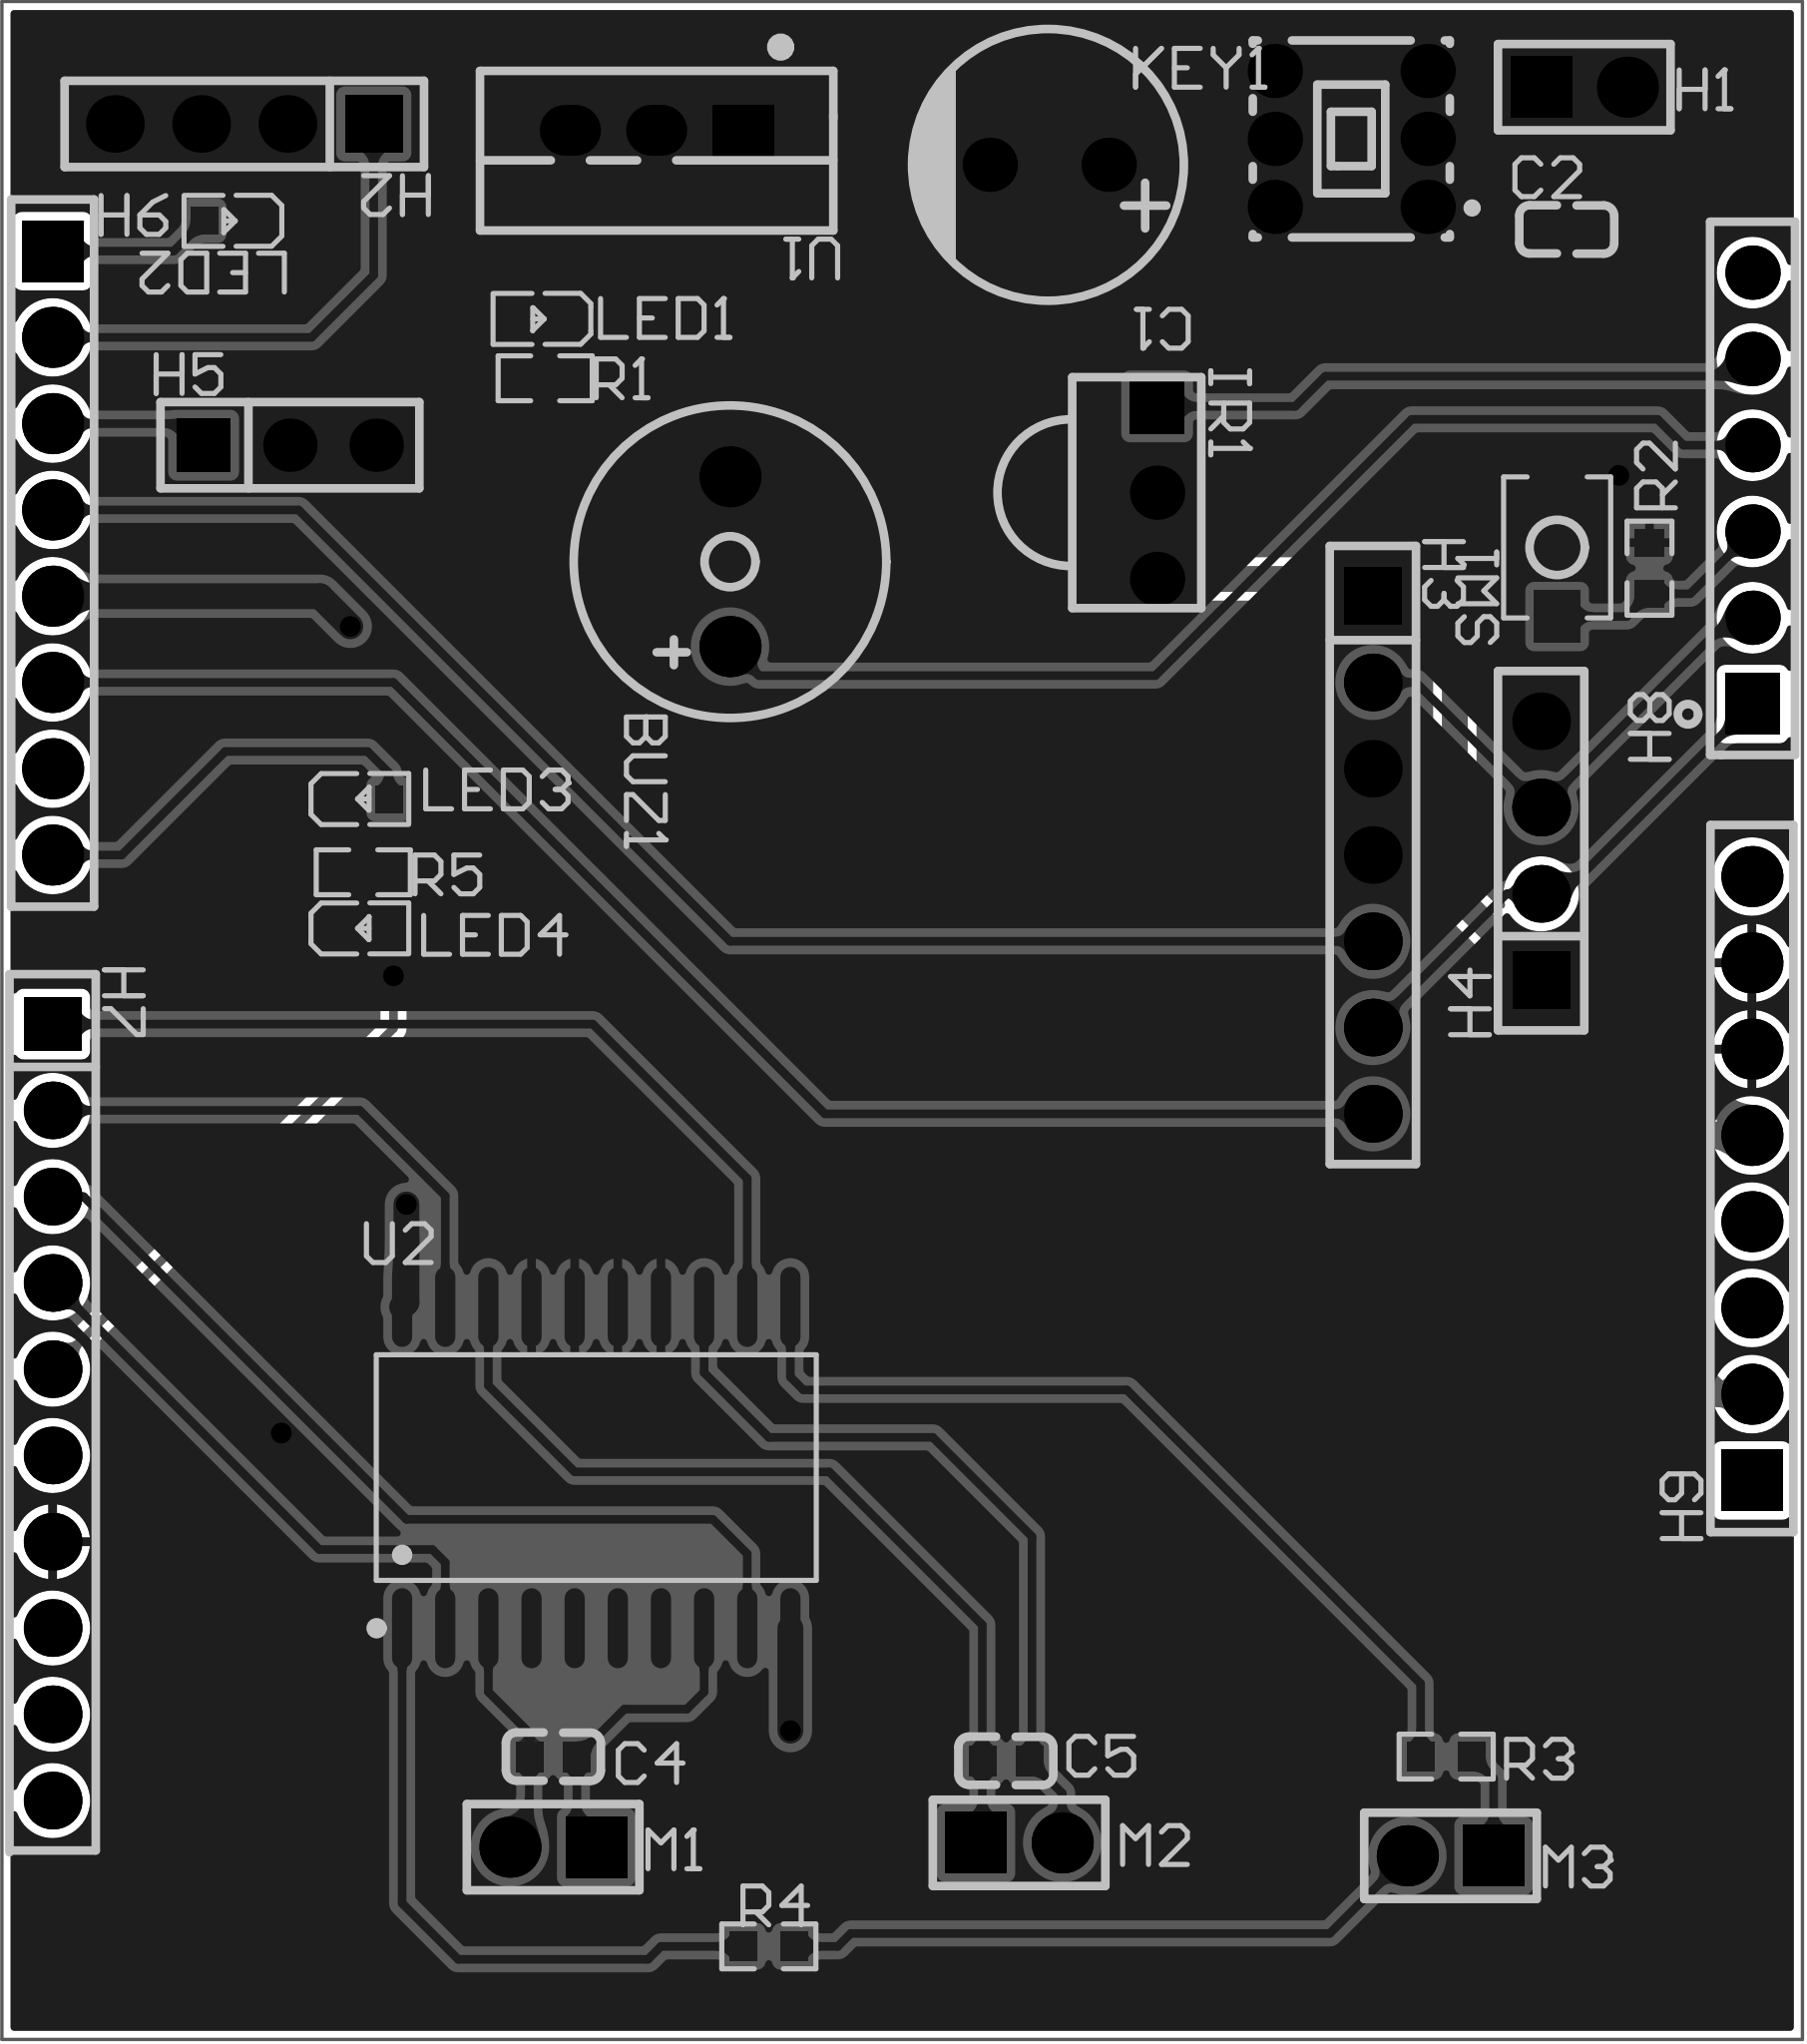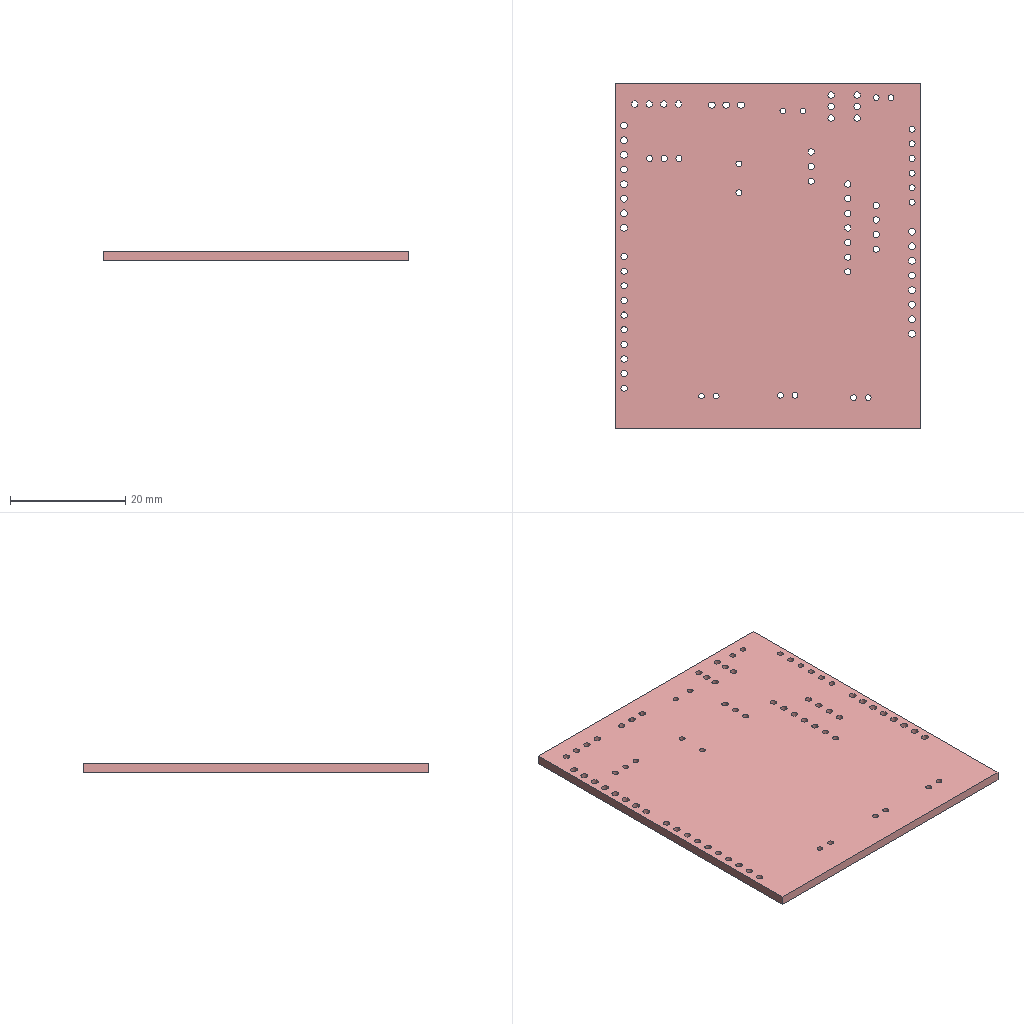Circuit board layout | Altium Designer | box 53 x 60 x 1.6 mm
Layer stack:
# Altium Designer layer stack of  (unit mm; dielectric type: 0 none, 1 core, 2 prepreg, 3 surface material)
index,name,kind,layer,copper_thickness_mm,dielectric_type,dielectric_thickness_mm,dielectric_material,dielectric_constant
0,Top Paste Mask Layer,other,,,,,,
1,Top Silkscreen Layer,other,,,,,,
2,Top Solder Mask Layer,dielectric,,,3,0.01,,3.3
3,Top Layer,copper,Top Layer,0.035,,,,
4,Dielectric1,dielectric,,,3,1.51,FR4,4.5
5,Bottom Layer,copper,Bottom Layer,0.035,,,,
6,Bottom Solder Mask Layer,dielectric,,,3,0.01,,3.3
7,Bottom Silkscreen Layer,other,,,,,,
8,Bottom Paste Mask Layer,other,,,,,,
# drill layer pairs: low layer,high layer
drill_pair,Top Layer,Bottom Layer
Part placement:
Designator,Comment,Layer,Footprint,Center-X(mm),Center-Y(mm),Rotation
BUZ1,蜂鸣器,TopLayer,BUZ-TH_BD9.0-P5.00-D0.6-FD,103.505,125.857,90
C1,1000uF,TopLayer,CAP-TH_BD8.0-P3.50-D0.6-FD,112.903,137.541,180
C2,100nF,TopLayer,C0603,128.143,135.636,0
C4,100nF,TopLayer,C0603,98.298,90.678,180
C5,100nF,TopLayer,C0603,111.633,90.551,0
H1,,TopLayer,HDR-TH_2P-P2.54-V-M-1,128.651,139.827,0
H2,,TopLayer,HDR-TH_4P-P2.54-V-F,89.208,138.745,180
H3,,TopLayer,HDR-TH_7P-P2.54-V-M,122.428,117.221,270
H4,,TopLayer,HDR-TH_4P-P2.54-V-F,127.381,117.348,90
H5,,TopLayer,HDR-TH_3P-P2.54-V-F,90.551,129.286,0
H6,,TopLayer,HDR-TH_8P-P2.54-V-F-1,83.566,126.111,270
H7,,TopLayer,HDR-TH_10P-P2.54-V-F,83.566,100.813,270
H8,,TopLayer,HDR-TH_6P-P2.54-V-F,133.604,128.016,90
H9,,TopLayer,HDR-TH_8P-P2.54-V-F-1,133.585,107.696,90
IR1,IRM-8601M2(GPS),TopLayer,SENSOR-TH_IRM-8601,116.078,127.889,270
KEY1,自锁开关 5.8Z白灰白260G,TopLayer,SW-TH_6P-L5.8-W5.8-P2.00-LS4.5-TR,121.793,138.303,270
LED1,,TopLayer,LED_0603,97.92,133.011,180
LED2,,TopLayer,LED_0603,88.824,135.898,180
LED3,,TopLayer,LED_0603,92.659,118.864,0
LED4,,TopLayer,LED_0603,92.659,115.054,0
M1,,TopLayer,HDR-TH_2P-P2.54-V-M-1,98.298,88.011,180
M2,,TopLayer,HDR-TH_2P-P2.54-V-M-1,112.014,88.138,0
M3,,TopLayer,HDR-TH_2P-P2.54-V-M-1,124.714,87.757,180
R1,4.7K,TopLayer,R0603,98.065,131.257,0
R2,4.7K,TopLayer,R0603,130.571,125.666,270
R3,1K,TopLayer,R0603,124.587,90.678,0
R4,1K,TopLayer,R0603,104.648,85.09,0
R5,4.7K,TopLayer,R0603,92.71,116.713,0
SW1,,TopLayer,Key_SMD_3x4x2,127.853,126.277,90
U1,7805,TopLayer,TO-220-3_L10.2-W4.5-P2.54-L-1,101.346,138.557,180
U2,L293DD,TopLayer,SOIC-20_L13.0-W7.6-P1.27-LS10.3-BL,99.568,99.187,0
Pad and via stacks:
# Altium Designer via and pad stacks of  (unit mm). Each distinct definition once, with the count of objects using it.
# via: kind,start_layer,end_layer,hole_mm,diameter_mm,mode(0 simple;1 top-mid-bottom;2 full stack),diameter_per_layer,count,example_net
# pad: kind,layer,hole_mm,hole_type(0 round;1 square;2 slot),plating,top_size,top_shape(1 round;2 rect;3 octagon;9 rounded rect),mid_size,bottom_size,mode,footprint,size_per_layer,count,example
pad,Multi-Layer,1,0,plated,1.8x1.8,1,1.8x1.8,1.8x1.8,0,BUZ-TH_BD9.0-P5.00-D0.6-FD,,2,BUZ1.1
pad,Multi-Layer,1,0,plated,1.6x1.6,1,1.6x1.6,1.6x1.6,0,CAP-TH_BD8.0-P3.50-D0.6-FD,,2,C1.2
pad,Multi-Layer,1,0,plated,1.8x1.8,1,1.8x1.8,1.8x1.8,0,HDR-TH_2P-P2.54-V-M-1,,4,H1.2
pad,Multi-Layer,1,0,plated,1.8x1.8,2,1.8x1.8,1.8x1.8,0,HDR-TH_2P-P2.54-V-M-1,,4,H1.1
pad,Multi-Layer,1.1,0,plated,1.7x1.7,2,1.7x1.7,1.7x1.7,0,HDR-TH_4P-P2.54-V-F,,2,H2.1
pad,Multi-Layer,1.1,0,plated,1.7x1.7,1,1.7x1.7,1.7x1.7,0,HDR-TH_4P-P2.54-V-F,,6,H2.2
pad,Multi-Layer,1.1,0,plated,1.7x1.7,2,1.7x1.7,1.7x1.7,0,HDR-TH_7P-P2.54-V-M,,1,H3.1
pad,Multi-Layer,1.1,0,plated,1.7x1.7,1,1.7x1.7,1.7x1.7,0,HDR-TH_7P-P2.54-V-M,,6,H3.2
pad,Multi-Layer,1.02,0,plated,1.575x1.575,1,1.575x1.575,1.575x1.575,0,HDR-TH_3P-P2.54-V-F,,2,H5.3
pad,Multi-Layer,1.02,0,plated,1.575x1.575,2,1.575x1.575,1.575x1.575,0,HDR-TH_3P-P2.54-V-F,,1,H5.1
pad,Multi-Layer,1.2,0,plated,1.8x1.8,2,1.8x1.8,1.8x1.8,0,HDR-TH_8P-P2.54-V-F-1,,2,H6.1
pad,Multi-Layer,1.2,0,plated,1.8x1.8,1,1.8x1.8,1.8x1.8,0,HDR-TH_8P-P2.54-V-F-1,,14,H6.2
pad,Multi-Layer,1.1,0,plated,1.7x1.7,1,1.7x1.7,1.7x1.7,0,HDR-TH_10P-P2.54-V-F,,9,H7.10
pad,Multi-Layer,1.1,0,plated,1.575x1.7,2,1.575x1.7,1.575x1.7,0,HDR-TH_10P-P2.54-V-F,,1,H7.1
pad,Multi-Layer,1.02,0,plated,1.6x1.6,1,1.6x1.6,1.6x1.6,0,HDR-TH_6P-P2.54-V-F,,5,H8.6
pad,Multi-Layer,1.02,0,plated,1.8x1.6,2,1.8x1.6,1.8x1.6,0,HDR-TH_6P-P2.54-V-F,,1,H8.1
pad,Multi-Layer,1.1,0,plated,1.6x1.6,2,1.6x1.6,1.6x1.6,0,SENSOR-TH_IRM-8601,,1,IR1.1
pad,Multi-Layer,1.1,0,plated,1.6x1.6,1,1.6x1.6,1.6x1.6,0,SENSOR-TH_IRM-8601,,2,IR1.2
pad,Multi-Layer,1.1,0,plated,1.6x1.6,1,1.6x1.6,1.6x1.6,0,SW-TH_6P-L5.8-W5.8-P2.00-LS4.5-TR,,6,KEY1.6
pad,Multi-Layer,1,2,plated,1.8x1.5,2,1.8x1.5,1.8x1.5,0,TO-220-3_L10.2-W4.5-P2.54-L-1,,1,U1.1
pad,Multi-Layer,1,2,plated,1.8x1.5,1,1.8x1.5,1.8x1.5,0,TO-220-3_L10.2-W4.5-P2.54-L-1,,2,U1.3
pad,Top Layer,0,0,plated,0.8x0.9,2,0.8x0.9,0.8x0.9,0,C0603,,6,C2.2
pad,Top Layer,0,0,plated,0.8001x0.8001,2,0.8001x0.8001,0.8001x0.8001,0,LED_0603,,8,LED1.1
pad,Top Layer,0,0,plated,0.8065x0.864,2,0.8065x0.864,0.8065x0.864,0,R0603,,10,R1.2
pad,Top Layer,0,0,plated,1.53x1.36,2,1.53x1.36,1.53x1.36,0,Key_SMD_3x4x2,,2,SW1.1
pad,Top Layer,0,0,plated,0.595x2.36,1,0.595x2.36,0.595x2.36,0,SOIC-20_L13.0-W7.6-P1.27-LS10.3-BL,,20,U2.1
via,Top Layer,Bottom Layer,0.3048,0.6096,0,,5,$1N3068
via,Top Layer,Bottom Layer,0.3048,0.61,0,,1,GND
Copper pours:
name,layer,net,type(0 solid;1 hatched;2 none)
Top Layer-GND,Top Layer,GND,0
Bottom Layer-GND,Bottom Layer,GND,0